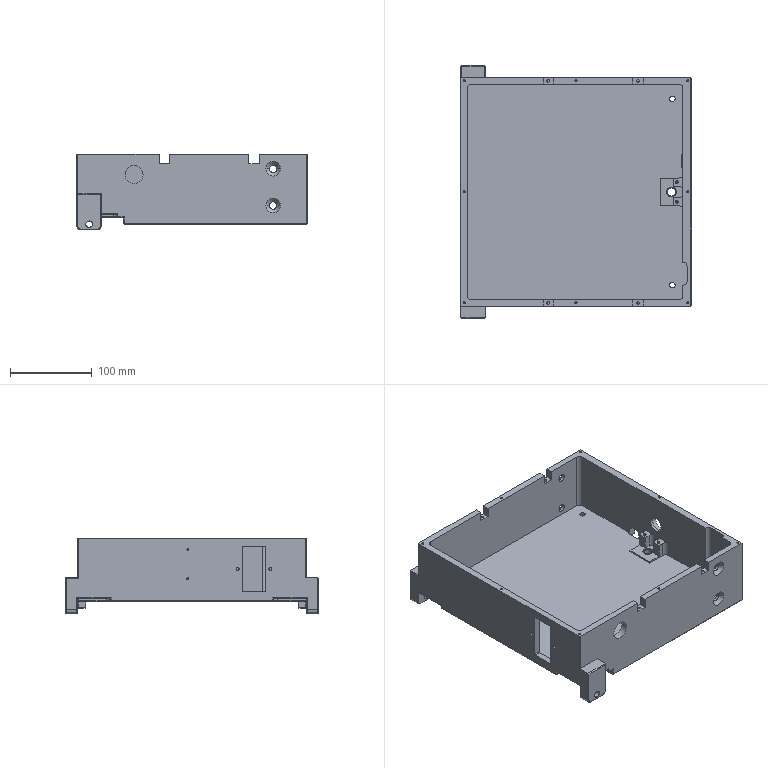NC program | Mastercam | posted with a generic post
Lines 1 to 46 of 104433:
%
:0001()
(MATERIAL - ALUMINUM MM - 2024)
(T24|100 FEM |H24)
(T23|50 FEM |H23|XY STOCK TO LEAVE - .5|Z STOCK TO LEAVE - .1)
(T20|20 FEM |H20)
(T10|10 FEM |H10|XY STOCK TO LEAVE - .1|Z STOCK TO LEAVE - .1)
(T11|10 FEM |H11)
(T1|6 CHM |H1)
(T7|6 CHM |H7)
(T2|2 FEM |H2|XY STOCK TO LEAVE - .03|Z STOCK TO LEAVE - 0.)
(T6|6 FEM |H6|XY STOCK TO LEAVE - .1|Z STOCK TO LEAVE - .1)
(T12|12 FEM |H12|XY STOCK TO LEAVE - .1|Z STOCK TO LEAVE - .1)
(T5|5 FEM |H5|XY STOCK TO LEAVE - .07|Z STOCK TO LEAVE - 0.)
(T15|6 BNOS |H15)
(T4|4 BM/BNOS |H4)
N100 G21
N102 G0 G17 G40 G80 G90 G94 G98
N104 G0 G28 G91 Z0.
N106 G0 G28 X0. Y0.
(100 FEM |TOOL - 24|DIA. OFF. - 24|LEN. - 24|TOOL DIA. - 100.)
N108 T24 M6
N110 G0 G54 G90 X-270. Y114.998 C0. B0. S4000 M3
N112 G43 H24 Z50.
N114 Z2.
N116 G1 Z0. F600.
N118 X210. F1200.
N120 G2 X238.749 Y86.249 J-28.749
N122 X210. Y57.499 I-28.749
N124 G1 X-210.
N126 G3 X-238.749 Y28.75 J-28.749
N128 X-210. Y0. I28.749
N130 G1 X210.
N132 G2 X238.75 Y-28.75 J-28.75
N134 X210. Y-57.499 I-28.75
N136 G1 X-210.
N138 G3 X-238.75 Y-86.249 J-28.75
N140 X-210. Y-114.998 I28.75
N142 G1 X270.
N144 G0 Z50.
N146 M5
N148 G0 G28 G91 Z0.
N150 G28
N152 M01
N154 G0 G17 G40 G80 G90 G94 G98
N156 G0 G28 G91 Z0.